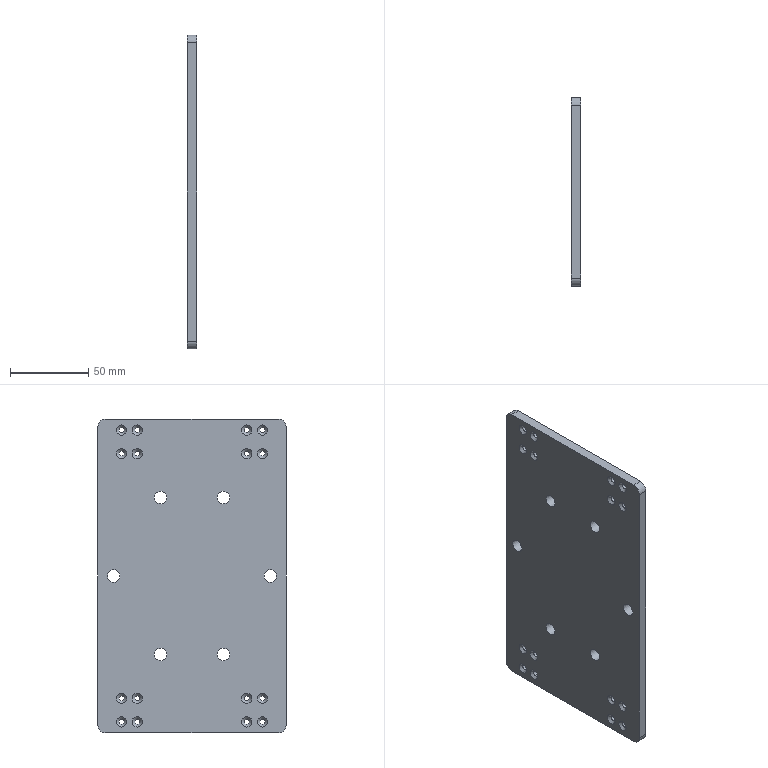Part | STEP file | JBJ-P-1014-02 | 1 solid | 48 faces | box 6 x 120 x 200 mm | volume 140903 mm3 | cylinder 26 | cone 16 | plane 6 | commonest cylinder face diameters 3.4 x16 8 x6 10 x4
STEP:
#1=CARTESIAN_POINT('',(0.,-110.,-96.));
#2=VERTEX_POINT('',#1);
#3=CARTESIAN_POINT('',(0.,-110.,-100.));
#4=DIRECTION('',(-1.,0.,0.));
#5=DIRECTION('',(0.,0.,1.));
#6=AXIS2_PLACEMENT_3D('',#3,#4,#5);
#7=CIRCLE('',#6,4.);
#8=EDGE_CURVE('',#2,#2,#7,.T.);
#9=ORIENTED_EDGE('',*,*,#8,.F.);
#10=EDGE_LOOP('',(#9));
#11=FACE_BOUND('',#10,.T.);
#12=CARTESIAN_POINT('',(0.,-80.,-46.));
#13=VERTEX_POINT('',#12);
#14=CARTESIAN_POINT('',(0.,-80.,-50.));
#15=DIRECTION('',(-1.,0.,0.));
#16=DIRECTION('',(0.,0.,1.));
#17=AXIS2_PLACEMENT_3D('',#14,#15,#16);
#18=CIRCLE('',#17,4.);
#19=EDGE_CURVE('',#13,#13,#18,.T.);
#20=ORIENTED_EDGE('',*,*,#19,.F.);
#21=EDGE_LOOP('',(#20));
#22=FACE_BOUND('',#21,.T.);
#23=CARTESIAN_POINT('',(0.,-40.,-46.));
#24=VERTEX_POINT('',#23);
#25=CARTESIAN_POINT('',(0.,-40.,-50.));
#26=DIRECTION('',(-1.,0.,0.));
#27=DIRECTION('',(0.,0.,1.));
#28=AXIS2_PLACEMENT_3D('',#25,#26,#27);
#29=CIRCLE('',#28,4.);
#30=EDGE_CURVE('',#24,#24,#29,.T.);
#31=ORIENTED_EDGE('',*,*,#30,.F.);
#32=EDGE_LOOP('',(#31));
#33=FACE_BOUND('',#32,.T.);
#34=CARTESIAN_POINT('',(0.,-40.,-146.));
#35=VERTEX_POINT('',#34);
#36=CARTESIAN_POINT('',(0.,-40.,-150.));
#37=DIRECTION('',(-1.,0.,0.));
#38=DIRECTION('',(0.,0.,1.));
#39=AXIS2_PLACEMENT_3D('',#36,#37,#38);
#40=CIRCLE('',#39,4.);
#41=EDGE_CURVE('',#35,#35,#40,.T.);
#42=ORIENTED_EDGE('',*,*,#41,.F.);
#43=EDGE_LOOP('',(#42));
#44=FACE_BOUND('',#43,.T.);
#45=CARTESIAN_POINT('',(0.,-80.,-146.));
#46=VERTEX_POINT('',#45);
#47=CARTESIAN_POINT('',(0.,-80.,-150.));
#48=DIRECTION('',(-1.,0.,0.));
#49=DIRECTION('',(0.,0.,1.));
#50=AXIS2_PLACEMENT_3D('',#47,#48,#49);
#51=CIRCLE('',#50,4.);
#52=EDGE_CURVE('',#46,#46,#51,.T.);
#53=ORIENTED_EDGE('',*,*,#52,.F.);
#54=EDGE_LOOP('',(#53));
#55=FACE_BOUND('',#54,.T.);
#56=CARTESIAN_POINT('',(0.,-104.9,-18.7));
#57=VERTEX_POINT('',#56);
#58=CARTESIAN_POINT('',(0.,-104.9,-22.));
#59=DIRECTION('',(-1.,0.,0.));
#60=DIRECTION('',(0.,0.,1.));
#61=AXIS2_PLACEMENT_3D('',#58,#59,#60);
#62=CIRCLE('',#61,3.3);
#63=EDGE_CURVE('',#57,#57,#62,.T.);
#64=ORIENTED_EDGE('',*,*,#63,.F.);
#65=EDGE_LOOP('',(#64));
#66=FACE_BOUND('',#65,.T.);
#67=CARTESIAN_POINT('',(0.,-104.9,-3.7));
#68=VERTEX_POINT('',#67);
#69=CARTESIAN_POINT('',(0.,-104.9,-7.));
#70=DIRECTION('',(-1.,0.,0.));
#71=DIRECTION('',(0.,0.,1.));
#72=AXIS2_PLACEMENT_3D('',#69,#70,#71);
#73=CIRCLE('',#72,3.3);
#74=EDGE_CURVE('',#68,#68,#73,.T.);
#75=ORIENTED_EDGE('',*,*,#74,.F.);
#76=EDGE_LOOP('',(#75));
#77=FACE_BOUND('',#76,.T.);
#78=CARTESIAN_POINT('',(0.,-94.9,-3.7));
#79=VERTEX_POINT('',#78);
#80=CARTESIAN_POINT('',(0.,-94.9,-7.));
#81=DIRECTION('',(-1.,0.,0.));
#82=DIRECTION('',(0.,0.,1.));
#83=AXIS2_PLACEMENT_3D('',#80,#81,#82);
#84=CIRCLE('',#83,3.3);
#85=EDGE_CURVE('',#79,#79,#84,.T.);
#86=ORIENTED_EDGE('',*,*,#85,.F.);
#87=EDGE_LOOP('',(#86));
#88=FACE_BOUND('',#87,.T.);
#89=CARTESIAN_POINT('',(0.,-25.1,-3.7));
#90=VERTEX_POINT('',#89);
#91=CARTESIAN_POINT('',(0.,-25.1,-7.));
#92=DIRECTION('',(-1.,0.,0.));
#93=DIRECTION('',(0.,0.,1.));
#94=AXIS2_PLACEMENT_3D('',#91,#92,#93);
#95=CIRCLE('',#94,3.3);
#96=EDGE_CURVE('',#90,#90,#95,.T.);
#97=ORIENTED_EDGE('',*,*,#96,.F.);
#98=EDGE_LOOP('',(#97));
#99=FACE_BOUND('',#98,.T.);
#100=CARTESIAN_POINT('',(0.,-15.1,-3.7));
#101=VERTEX_POINT('',#100);
#102=CARTESIAN_POINT('',(0.,-15.1,-7.));
#103=DIRECTION('',(-1.,0.,0.));
#104=DIRECTION('',(0.,0.,1.));
#105=AXIS2_PLACEMENT_3D('',#102,#103,#104);
#106=CIRCLE('',#105,3.3);
#107=EDGE_CURVE('',#101,#101,#106,.T.);
#108=ORIENTED_EDGE('',*,*,#107,.F.);
#109=EDGE_LOOP('',(#108));
#110=FACE_BOUND('',#109,.T.);
#111=CARTESIAN_POINT('',(0.,-25.1,-18.7));
#112=VERTEX_POINT('',#111);
#113=CARTESIAN_POINT('',(0.,-25.1,-22.));
#114=DIRECTION('',(-1.,0.,0.));
#115=DIRECTION('',(0.,0.,1.));
#116=AXIS2_PLACEMENT_3D('',#113,#114,#115);
#117=CIRCLE('',#116,3.3);
#118=EDGE_CURVE('',#112,#112,#117,.T.);
#119=ORIENTED_EDGE('',*,*,#118,.F.);
#120=EDGE_LOOP('',(#119));
#121=FACE_BOUND('',#120,.T.);
#122=CARTESIAN_POINT('',(0.,-15.1,-18.7));
#123=VERTEX_POINT('',#122);
#124=CARTESIAN_POINT('',(0.,-15.1,-22.));
#125=DIRECTION('',(-1.,0.,0.));
#126=DIRECTION('',(0.,0.,1.));
#127=AXIS2_PLACEMENT_3D('',#124,#125,#126);
#128=CIRCLE('',#127,3.3);
#129=EDGE_CURVE('',#123,#123,#128,.T.);
#130=ORIENTED_EDGE('',*,*,#129,.F.);
#131=EDGE_LOOP('',(#130));
#132=FACE_BOUND('',#131,.T.);
#133=CARTESIAN_POINT('',(0.,-104.9,-174.7));
#134=VERTEX_POINT('',#133);
#135=CARTESIAN_POINT('',(0.,-104.9,-178.));
#136=DIRECTION('',(-1.,0.,0.));
#137=DIRECTION('',(0.,0.,1.));
#138=AXIS2_PLACEMENT_3D('',#135,#136,#137);
#139=CIRCLE('',#138,3.3);
#140=EDGE_CURVE('',#134,#134,#139,.T.);
#141=ORIENTED_EDGE('',*,*,#140,.F.);
#142=EDGE_LOOP('',(#141));
#143=FACE_BOUND('',#142,.T.);
#144=CARTESIAN_POINT('',(0.,-104.9,-189.7));
#145=VERTEX_POINT('',#144);
#146=CARTESIAN_POINT('',(0.,-104.9,-193.));
#147=DIRECTION('',(-1.,0.,0.));
#148=DIRECTION('',(0.,0.,1.));
#149=AXIS2_PLACEMENT_3D('',#146,#147,#148);
#150=CIRCLE('',#149,3.3);
#151=EDGE_CURVE('',#145,#145,#150,.T.);
#152=ORIENTED_EDGE('',*,*,#151,.F.);
#153=EDGE_LOOP('',(#152));
#154=FACE_BOUND('',#153,.T.);
#155=CARTESIAN_POINT('',(0.,-94.9,-189.7));
#156=VERTEX_POINT('',#155);
#157=CARTESIAN_POINT('',(0.,-94.9,-193.));
#158=DIRECTION('',(-1.,0.,0.));
#159=DIRECTION('',(0.,0.,1.));
#160=AXIS2_PLACEMENT_3D('',#157,#158,#159);
#161=CIRCLE('',#160,3.3);
#162=EDGE_CURVE('',#156,#156,#161,.T.);
#163=ORIENTED_EDGE('',*,*,#162,.F.);
#164=EDGE_LOOP('',(#163));
#165=FACE_BOUND('',#164,.T.);
#166=CARTESIAN_POINT('',(0.,-94.9,-174.7));
#167=VERTEX_POINT('',#166);
#168=CARTESIAN_POINT('',(0.,-94.9,-178.));
#169=DIRECTION('',(-1.,0.,0.));
#170=DIRECTION('',(0.,0.,1.));
#171=AXIS2_PLACEMENT_3D('',#168,#169,#170);
#172=CIRCLE('',#171,3.3);
#173=EDGE_CURVE('',#167,#167,#172,.T.);
#174=ORIENTED_EDGE('',*,*,#173,.F.);
#175=EDGE_LOOP('',(#174));
#176=FACE_BOUND('',#175,.T.);
#177=CARTESIAN_POINT('',(0.,-25.1,-174.7));
#178=VERTEX_POINT('',#177);
#179=CARTESIAN_POINT('',(0.,-25.1,-178.));
#180=DIRECTION('',(-1.,0.,0.));
#181=DIRECTION('',(0.,0.,1.));
#182=AXIS2_PLACEMENT_3D('',#179,#180,#181);
#183=CIRCLE('',#182,3.3);
#184=EDGE_CURVE('',#178,#178,#183,.T.);
#185=ORIENTED_EDGE('',*,*,#184,.F.);
#186=EDGE_LOOP('',(#185));
#187=FACE_BOUND('',#186,.T.);
#188=CARTESIAN_POINT('',(0.,-15.1,-174.7));
#189=VERTEX_POINT('',#188);
#190=CARTESIAN_POINT('',(0.,-15.1,-178.));
#191=DIRECTION('',(-1.,0.,0.));
#192=DIRECTION('',(0.,0.,1.));
#193=AXIS2_PLACEMENT_3D('',#190,#191,#192);
#194=CIRCLE('',#193,3.3);
#195=EDGE_CURVE('',#189,#189,#194,.T.);
#196=ORIENTED_EDGE('',*,*,#195,.F.);
#197=EDGE_LOOP('',(#196));
#198=FACE_BOUND('',#197,.T.);
#199=CARTESIAN_POINT('',(0.,-15.1,-189.7));
#200=VERTEX_POINT('',#199);
#201=CARTESIAN_POINT('',(0.,-15.1,-193.));
#202=DIRECTION('',(-1.,0.,0.));
#203=DIRECTION('',(0.,0.,1.));
#204=AXIS2_PLACEMENT_3D('',#201,#202,#203);
#205=CIRCLE('',#204,3.3);
#206=EDGE_CURVE('',#200,#200,#205,.T.);
#207=ORIENTED_EDGE('',*,*,#206,.F.);
#208=EDGE_LOOP('',(#207));
#209=FACE_BOUND('',#208,.T.);
#210=CARTESIAN_POINT('',(0.,-25.1,-189.7));
#211=VERTEX_POINT('',#210);
#212=CARTESIAN_POINT('',(0.,-25.1,-193.));
#213=DIRECTION('',(-1.,0.,0.));
#214=DIRECTION('',(0.,0.,1.));
#215=AXIS2_PLACEMENT_3D('',#212,#213,#214);
#216=CIRCLE('',#215,3.3);
#217=EDGE_CURVE('',#211,#211,#216,.T.);
#218=ORIENTED_EDGE('',*,*,#217,.F.);
#219=EDGE_LOOP('',(#218));
#220=FACE_BOUND('',#219,.T.);
#221=CARTESIAN_POINT('',(0.,-120.,-5.));
#222=VERTEX_POINT('',#221);
#223=CARTESIAN_POINT('',(0.,-120.,-195.));
#224=VERTEX_POINT('',#223);
#225=CARTESIAN_POINT('',(0.,-120.,0.));
#226=DIRECTION('',(0.,0.,-1.));
#227=VECTOR('',#226,1000.);
#228=LINE('',#225,#227);
#229=EDGE_CURVE('',#222,#224,#228,.T.);
#230=ORIENTED_EDGE('',*,*,#229,.F.);
#231=CARTESIAN_POINT('',(0.,-115.,0.));
#232=VERTEX_POINT('',#231);
#233=CARTESIAN_POINT('',(0.,-115.,-5.));
#234=DIRECTION('',(-1.,0.,0.));
#235=DIRECTION('',(0.,0.,-1.));
#236=AXIS2_PLACEMENT_3D('',#233,#234,#235);
#237=CIRCLE('',#236,5.);
#238=EDGE_CURVE('',#222,#232,#237,.T.);
#239=ORIENTED_EDGE('',*,*,#238,.T.);
#240=CARTESIAN_POINT('',(0.,-5.,0.));
#241=VERTEX_POINT('',#240);
#242=CARTESIAN_POINT('',(0.,0.,0.));
#243=DIRECTION('',(0.,-1.,0.));
#244=VECTOR('',#243,1000.);
#245=LINE('',#242,#244);
#246=EDGE_CURVE('',#241,#232,#245,.T.);
#247=ORIENTED_EDGE('',*,*,#246,.F.);
#248=CARTESIAN_POINT('',(0.,0.,-5.));
#249=VERTEX_POINT('',#248);
#250=CARTESIAN_POINT('',(0.,-5.,-5.));
#251=DIRECTION('',(-1.,0.,0.));
#252=DIRECTION('',(0.,0.,-1.));
#253=AXIS2_PLACEMENT_3D('',#250,#251,#252);
#254=CIRCLE('',#253,5.);
#255=EDGE_CURVE('',#241,#249,#254,.T.);
#256=ORIENTED_EDGE('',*,*,#255,.T.);
#257=CARTESIAN_POINT('',(0.,0.,-195.));
#258=VERTEX_POINT('',#257);
#259=CARTESIAN_POINT('',(0.,0.,0.));
#260=DIRECTION('',(0.,0.,1.));
#261=VECTOR('',#260,1000.);
#262=LINE('',#259,#261);
#263=EDGE_CURVE('',#258,#249,#262,.T.);
#264=ORIENTED_EDGE('',*,*,#263,.F.);
#265=CARTESIAN_POINT('',(0.,-5.,-200.));
#266=VERTEX_POINT('',#265);
#267=CARTESIAN_POINT('',(0.,-5.,-195.));
#268=DIRECTION('',(-1.,0.,0.));
#269=DIRECTION('',(0.,0.,-1.));
#270=AXIS2_PLACEMENT_3D('',#267,#268,#269);
#271=CIRCLE('',#270,5.);
#272=EDGE_CURVE('',#258,#266,#271,.T.);
#273=ORIENTED_EDGE('',*,*,#272,.T.);
#274=CARTESIAN_POINT('',(0.,-115.,-200.));
#275=VERTEX_POINT('',#274);
#276=CARTESIAN_POINT('',(0.,0.,-200.));
#277=DIRECTION('',(0.,1.,0.));
#278=VECTOR('',#277,1000.);
#279=LINE('',#276,#278);
#280=EDGE_CURVE('',#275,#266,#279,.T.);
#281=ORIENTED_EDGE('',*,*,#280,.F.);
#282=CARTESIAN_POINT('',(0.,-115.,-195.));
#283=DIRECTION('',(-1.,0.,0.));
#284=DIRECTION('',(0.,0.,-1.));
#285=AXIS2_PLACEMENT_3D('',#282,#283,#284);
#286=CIRCLE('',#285,5.);
#287=EDGE_CURVE('',#275,#224,#286,.T.);
#288=ORIENTED_EDGE('',*,*,#287,.T.);
#289=EDGE_LOOP('',(#230,#239,#247,#256,#264,#273,#281,#288));
#290=FACE_OUTER_BOUND('',#289,.T.);
#291=CARTESIAN_POINT('',(0.,-94.9,-18.7));
#292=VERTEX_POINT('',#291);
#293=CARTESIAN_POINT('',(0.,-94.9,-22.));
#294=DIRECTION('',(-1.,0.,0.));
#295=DIRECTION('',(0.,0.,1.));
#296=AXIS2_PLACEMENT_3D('',#293,#294,#295);
#297=CIRCLE('',#296,3.3);
#298=EDGE_CURVE('',#292,#292,#297,.T.);
#299=ORIENTED_EDGE('',*,*,#298,.F.);
#300=EDGE_LOOP('',(#299));
#301=FACE_BOUND('',#300,.T.);
#302=CARTESIAN_POINT('',(0.,-10.,-96.));
#303=VERTEX_POINT('',#302);
#304=CARTESIAN_POINT('',(0.,-10.,-100.));
#305=DIRECTION('',(-1.,0.,0.));
#306=DIRECTION('',(0.,0.,1.));
#307=AXIS2_PLACEMENT_3D('',#304,#305,#306);
#308=CIRCLE('',#307,4.);
#309=EDGE_CURVE('',#303,#303,#308,.T.);
#310=ORIENTED_EDGE('',*,*,#309,.F.);
#311=EDGE_LOOP('',(#310));
#312=FACE_BOUND('',#311,.T.);
#313=CARTESIAN_POINT('',(0.,0.,0.));
#314=DIRECTION('',(1.,0.,0.));
#315=DIRECTION('',(0.,0.,-1.));
#316=AXIS2_PLACEMENT_3D('',#313,#314,#315);
#317=PLANE('',#316);
#318=ADVANCED_FACE('',(#11,#22,#33,#44,#55,#66,#77,#88,#99,#110,#121,#132,#143,#154,#165,#176,#187,#198,#209,#220,#290,#301,#312),#317,.F.);
#319=ORIENTED_EDGE('',*,*,#246,.T.);
#320=CARTESIAN_POINT('',(6.,-115.,0.));
#321=VERTEX_POINT('',#320);
#322=CARTESIAN_POINT('',(6.,-115.,0.));
#323=DIRECTION('',(1.,0.,0.));
#324=VECTOR('',#323,1000.);
#325=LINE('',#322,#324);
#326=EDGE_CURVE('',#232,#321,#325,.T.);
#327=ORIENTED_EDGE('',*,*,#326,.T.);
#328=CARTESIAN_POINT('',(6.,-5.,0.));
#329=VERTEX_POINT('',#328);
#330=CARTESIAN_POINT('',(6.,0.,0.));
#331=DIRECTION('',(0.,-1.,0.));
#332=VECTOR('',#331,1000.);
#333=LINE('',#330,#332);
#334=EDGE_CURVE('',#329,#321,#333,.T.);
#335=ORIENTED_EDGE('',*,*,#334,.F.);
#336=CARTESIAN_POINT('',(6.,-5.,0.));
#337=DIRECTION('',(-1.,0.,0.));
#338=VECTOR('',#337,1000.);
#339=LINE('',#336,#338);
#340=EDGE_CURVE('',#329,#241,#339,.T.);
#341=ORIENTED_EDGE('',*,*,#340,.T.);
#342=EDGE_LOOP('',(#319,#327,#335,#341));
#343=FACE_OUTER_BOUND('',#342,.T.);
#344=CARTESIAN_POINT('',(6.,0.,0.));
#345=DIRECTION('',(0.,0.,-1.));
#346=DIRECTION('',(0.,1.,0.));
#347=AXIS2_PLACEMENT_3D('',#344,#345,#346);
#348=PLANE('',#347);
#349=ADVANCED_FACE('',(#343),#348,.F.);
#350=CARTESIAN_POINT('',(6.,-120.,-5.));
#351=VERTEX_POINT('',#350);
#352=CARTESIAN_POINT('',(6.,-120.,-195.));
#353=VERTEX_POINT('',#352);
#354=CARTESIAN_POINT('',(6.,-120.,0.));
#355=DIRECTION('',(0.,0.,-1.));
#356=VECTOR('',#355,1000.);
#357=LINE('',#354,#356);
#358=EDGE_CURVE('',#351,#353,#357,.T.);
#359=ORIENTED_EDGE('',*,*,#358,.F.);
#360=CARTESIAN_POINT('',(6.,-120.,-5.));
#361=DIRECTION('',(-1.,0.,0.));
#362=VECTOR('',#361,1000.);
#363=LINE('',#360,#362);
#364=EDGE_CURVE('',#351,#222,#363,.T.);
#365=ORIENTED_EDGE('',*,*,#364,.T.);
#366=ORIENTED_EDGE('',*,*,#229,.T.);
#367=CARTESIAN_POINT('',(6.,-120.,-195.));
#368=DIRECTION('',(1.,0.,0.));
#369=VECTOR('',#368,1000.);
#370=LINE('',#367,#369);
#371=EDGE_CURVE('',#224,#353,#370,.T.);
#372=ORIENTED_EDGE('',*,*,#371,.T.);
#373=EDGE_LOOP('',(#359,#365,#366,#372));
#374=FACE_OUTER_BOUND('',#373,.T.);
#375=CARTESIAN_POINT('',(6.,-120.,0.));
#376=DIRECTION('',(0.,1.,0.));
#377=DIRECTION('',(0.,0.,1.));
#378=AXIS2_PLACEMENT_3D('',#375,#376,#377);
#379=PLANE('',#378);
#380=ADVANCED_FACE('',(#374),#379,.F.);
#381=CARTESIAN_POINT('',(6.,-115.,-200.));
#382=VERTEX_POINT('',#381);
#383=CARTESIAN_POINT('',(6.,-5.,-200.));
#384=VERTEX_POINT('',#383);
#385=CARTESIAN_POINT('',(6.,0.,-200.));
#386=DIRECTION('',(0.,1.,0.));
#387=VECTOR('',#386,1000.);
#388=LINE('',#385,#387);
#389=EDGE_CURVE('',#382,#384,#388,.T.);
#390=ORIENTED_EDGE('',*,*,#389,.F.);
#391=CARTESIAN_POINT('',(6.,-115.,-200.));
#392=DIRECTION('',(-1.,0.,0.));
#393=VECTOR('',#392,1000.);
#394=LINE('',#391,#393);
#395=EDGE_CURVE('',#382,#275,#394,.T.);
#396=ORIENTED_EDGE('',*,*,#395,.T.);
#397=ORIENTED_EDGE('',*,*,#280,.T.);
#398=CARTESIAN_POINT('',(6.,-5.,-200.));
#399=DIRECTION('',(1.,0.,0.));
#400=VECTOR('',#399,1000.);
#401=LINE('',#398,#400);
#402=EDGE_CURVE('',#266,#384,#401,.T.);
#403=ORIENTED_EDGE('',*,*,#402,.T.);
#404=EDGE_LOOP('',(#390,#396,#397,#403));
#405=FACE_OUTER_BOUND('',#404,.T.);
#406=CARTESIAN_POINT('',(6.,0.,-200.));
#407=DIRECTION('',(0.,0.,1.));
#408=DIRECTION('',(0.,-1.,0.));
#409=AXIS2_PLACEMENT_3D('',#406,#407,#408);
#410=PLANE('',#409);
#411=ADVANCED_FACE('',(#405),#410,.F.);
#412=CARTESIAN_POINT('',(6.,0.,-195.));
#413=VERTEX_POINT('',#412);
#414=CARTESIAN_POINT('',(6.,0.,-5.));
#415=VERTEX_POINT('',#414);
#416=CARTESIAN_POINT('',(6.,0.,0.));
#417=DIRECTION('',(0.,0.,1.));
#418=VECTOR('',#417,1000.);
#419=LINE('',#416,#418);
#420=EDGE_CURVE('',#413,#415,#419,.T.);
#421=ORIENTED_EDGE('',*,*,#420,.F.);
#422=CARTESIAN_POINT('',(6.,0.,-195.));
#423=DIRECTION('',(-1.,0.,0.));
#424=VECTOR('',#423,1000.);
#425=LINE('',#422,#424);
#426=EDGE_CURVE('',#413,#258,#425,.T.);
#427=ORIENTED_EDGE('',*,*,#426,.T.);
#428=ORIENTED_EDGE('',*,*,#263,.T.);
#429=CARTESIAN_POINT('',(6.,0.,-5.));
#430=DIRECTION('',(1.,0.,0.));
#431=VECTOR('',#430,1000.);
#432=LINE('',#429,#431);
#433=EDGE_CURVE('',#249,#415,#432,.T.);
#434=ORIENTED_EDGE('',*,*,#433,.T.);
#435=EDGE_LOOP('',(#421,#427,#428,#434));
#436=FACE_OUTER_BOUND('',#435,.T.);
#437=CARTESIAN_POINT('',(6.,0.,0.));
#438=DIRECTION('',(0.,-1.,0.));
#439=DIRECTION('',(0.,0.,-1.));
#440=AXIS2_PLACEMENT_3D('',#437,#438,#439);
#441=PLANE('',#440);
#442=ADVANCED_FACE('',(#436),#441,.F.);
#443=CARTESIAN_POINT('',(6.,-10.,-96.));
#444=VERTEX_POINT('',#443);
#445=CARTESIAN_POINT('',(6.,-10.,-100.));
#446=DIRECTION('',(-1.,0.,0.));
#447=DIRECTION('',(0.,0.,1.));
#448=AXIS2_PLACEMENT_3D('',#445,#446,#447);
#449=CIRCLE('',#448,4.);
#450=EDGE_CURVE('',#444,#444,#449,.T.);
#451=ORIENTED_EDGE('',*,*,#450,.T.);
#452=EDGE_LOOP('',(#451));
#453=FACE_BOUND('',#452,.T.);
#454=CARTESIAN_POINT('',(6.,-110.,-96.));
#455=VERTEX_POINT('',#454);
#456=CARTESIAN_POINT('',(6.,-110.,-100.));
#457=DIRECTION('',(-1.,0.,0.));
#458=DIRECTION('',(0.,0.,1.));
#459=AXIS2_PLACEMENT_3D('',#456,#457,#458);
#460=CIRCLE('',#459,4.);
#461=EDGE_CURVE('',#455,#455,#460,.T.);
#462=ORIENTED_EDGE('',*,*,#461,.T.);
#463=EDGE_LOOP('',(#462));
#464=FACE_BOUND('',#463,.T.);
#465=CARTESIAN_POINT('',(6.,-80.,-46.));
#466=VERTEX_POINT('',#465);
#467=CARTESIAN_POINT('',(6.,-80.,-50.));
#468=DIRECTION('',(-1.,0.,0.));
#469=DIRECTION('',(0.,0.,1.));
#470=AXIS2_PLACEMENT_3D('',#467,#468,#469);
#471=CIRCLE('',#470,4.);
#472=EDGE_CURVE('',#466,#466,#471,.T.);
#473=ORIENTED_EDGE('',*,*,#472,.T.);
#474=EDGE_LOOP('',(#473));
#475=FACE_BOUND('',#474,.T.);
#476=CARTESIAN_POINT('',(6.,-40.,-46.));
#477=VERTEX_POINT('',#476);
#478=CARTESIAN_POINT('',(6.,-40.,-50.));
#479=DIRECTION('',(-1.,0.,0.));
#480=DIRECTION('',(0.,0.,1.));
#481=AXIS2_PLACEMENT_3D('',#478,#479,#480);
#482=CIRCLE('',#481,4.);
#483=EDGE_CURVE('',#477,#477,#482,.T.);
#484=ORIENTED_EDGE('',*,*,#483,.T.);
#485=EDGE_LOOP('',(#484));
#486=FACE_BOUND('',#485,.T.);
#487=CARTESIAN_POINT('',(6.,-40.,-146.));
#488=VERTEX_POINT('',#487);
#489=CARTESIAN_POINT('',(6.,-40.,-150.));
#490=DIRECTION('',(-1.,0.,0.));
#491=DIRECTION('',(0.,0.,1.));
#492=AXIS2_PLACEMENT_3D('',#489,#490,#491);
#493=CIRCLE('',#492,4.);
#494=EDGE_CURVE('',#488,#488,#493,.T.);
#495=ORIENTED_EDGE('',*,*,#494,.T.);
#496=EDGE_LOOP('',(#495));
#497=FACE_BOUND('',#496,.T.);
#498=CARTESIAN_POINT('',(6.,-80.,-146.));
#499=VERTEX_POINT('',#498);
#500=CARTESIAN_POINT('',(6.,-80.,-150.));
#501=DIRECTION('',(-1.,0.,0.));
#502=DIRECTION('',(0.,0.,1.));
#503=AXIS2_PLACEMENT_3D('',#500,#501,#502);
#504=CIRCLE('',#503,4.);
#505=EDGE_CURVE('',#499,#499,#504,.T.);
#506=ORIENTED_EDGE('',*,*,#505,.T.);
#507=EDGE_LOOP('',(#506));
#508=FACE_BOUND('',#507,.T.);
#509=CARTESIAN_POINT('',(6.,-104.9,-20.3));
#510=VERTEX_POINT('',#509);
#511=CARTESIAN_POINT('',(6.,-104.9,-22.));
#512=DIRECTION('',(-1.,0.,0.));
#513=DIRECTION('',(0.,0.,1.));
#514=AXIS2_PLACEMENT_3D('',#511,#512,#513);
#515=CIRCLE('',#514,1.7);
#516=EDGE_CURVE('',#510,#510,#515,.T.);
#517=ORIENTED_EDGE('',*,*,#516,.T.);
#518=EDGE_LOOP('',(#517));
#519=FACE_BOUND('',#518,.T.);
#520=CARTESIAN_POINT('',(6.,-104.9,-5.3));
#521=VERTEX_POINT('',#520);
#522=CARTESIAN_POINT('',(6.,-104.9,-7.));
#523=DIRECTION('',(-1.,0.,0.));
#524=DIRECTION('',(0.,0.,1.));
#525=AXIS2_PLACEMENT_3D('',#522,#523,#524);
#526=CIRCLE('',#525,1.7);
#527=EDGE_CURVE('',#521,#521,#526,.T.);
#528=ORIENTED_EDGE('',*,*,#527,.T.);
#529=EDGE_LOOP('',(#528));
#530=FACE_BOUND('',#529,.T.);
#531=CARTESIAN_POINT('',(6.,-94.9,-5.3));
#532=VERTEX_POINT('',#531);
#533=CARTESIAN_POINT('',(6.,-94.9,-7.));
#534=DIRECTION('',(-1.,0.,0.));
#535=DIRECTION('',(0.,0.,1.));
#536=AXIS2_PLACEMENT_3D('',#533,#534,#535);
#537=CIRCLE('',#536,1.7);
#538=EDGE_CURVE('',#532,#532,#537,.T.);
#539=ORIENTED_EDGE('',*,*,#538,.T.);
#540=EDGE_LOOP('',(#539));
#541=FACE_BOUND('',#540,.T.);
#542=CARTESIAN_POINT('',(6.,-94.9,-20.3));
#543=VERTEX_POINT('',#542);
#544=CARTESIAN_POINT('',(6.,-94.9,-22.));
#545=DIRECTION('',(-1.,0.,0.));
#546=DIRECTION('',(0.,0.,1.));
#547=AXIS2_PLACEMENT_3D('',#544,#545,#546);
#548=CIRCLE('',#547,1.7);
#549=EDGE_CURVE('',#543,#543,#548,.T.);
#550=ORIENTED_EDGE('',*,*,#549,.T.);
#551=EDGE_LOOP('',(#550));
#552=FACE_BOUND('',#551,.T.);
#553=CARTESIAN_POINT('',(6.,-25.1,-5.3));
#554=VERTEX_POINT('',#553);
#555=CARTESIAN_POINT('',(6.,-25.1,-7.));
#556=DIRECTION('',(-1.,0.,0.));
#557=DIRECTION('',(0.,0.,1.));
#558=AXIS2_PLACEMENT_3D('',#555,#556,#557);
#559=CIRCLE('',#558,1.7);
#560=EDGE_CURVE('',#554,#554,#559,.T.);
#561=ORIENTED_EDGE('',*,*,#560,.T.);
#562=EDGE_LOOP('',(#561));
#563=FACE_BOUND('',#562,.T.);
#564=CARTESIAN_POINT('',(6.,-15.1,-5.3));
#565=VERTEX_POINT('',#564);
#566=CARTESIAN_POINT('',(6.,-15.1,-7.));
#567=DIRECTION('',(-1.,0.,0.));
#568=DIRECTION('',(0.,0.,1.));
#569=AXIS2_PLACEMENT_3D('',#566,#567,#568);
#570=CIRCLE('',#569,1.7);
#571=EDGE_CURVE('',#565,#565,#570,.T.);
#572=ORIENTED_EDGE('',*,*,#571,.T.);
#573=EDGE_LOOP('',(#572));
#574=FACE_BOUND('',#573,.T.);
#575=CARTESIAN_POINT('',(6.,-25.1,-20.3));
#576=VERTEX_POINT('',#575);
#577=CARTESIAN_POINT('',(6.,-25.1,-22.));
#578=DIRECTION('',(-1.,0.,0.));
#579=DIRECTION('',(0.,0.,1.));
#580=AXIS2_PLACEMENT_3D('',#577,#578,#579);
#581=CIRCLE('',#580,1.7);
#582=EDGE_CURVE('',#576,#576,#581,.T.);
#583=ORIENTED_EDGE('',*,*,#582,.T.);
#584=EDGE_LOOP('',(#583));
#585=FACE_BOUND('',#584,.T.);
#586=CARTESIAN_POINT('',(6.,-15.1,-20.3));
#587=VERTEX_POINT('',#586);
#588=CARTESIAN_POINT('',(6.,-15.1,-22.));
#589=DIRECTION('',(-1.,0.,0.));
#590=DIRECTION('',(0.,0.,1.));
#591=AXIS2_PLACEMENT_3D('',#588,#589,#590);
#592=CIRCLE('',#591,1.7);
#593=EDGE_CURVE('',#587,#587,#592,.T.);
#594=ORIENTED_EDGE('',*,*,#593,.T.);
#595=EDGE_LOOP('',(#594));
#596=FACE_BOUND('',#595,.T.);
#597=CARTESIAN_POINT('',(6.,-104.9,-176.3));
#598=VERTEX_POINT('',#597);
#599=CARTESIAN_POINT('',(6.,-104.9,-178.));
#600=DIRECTION('',(-1.,0.,0.));
#601=DIRECTION('',(0.,0.,1.));
#602=AXIS2_PLACEMENT_3D('',#599,#600,#601);
#603=CIRCLE('',#602,1.7);
#604=EDGE_CURVE('',#598,#598,#603,.T.);
#605=ORIENTED_EDGE('',*,*,#604,.T.);
#606=EDGE_LOOP('',(#605));
#607=FACE_BOUND('',#606,.T.);
#608=CARTESIAN_POINT('',(6.,-104.9,-191.3));
#609=VERTEX_POINT('',#608);
#610=CARTESIAN_POINT('',(6.,-104.9,-193.));
#611=DIRECTION('',(-1.,0.,0.));
#612=DIRECTION('',(0.,0.,1.));
#613=AXIS2_PLACEMENT_3D('',#610,#611,#612);
#614=CIRCLE('',#613,1.7);
#615=EDGE_CURVE('',#609,#609,#614,.T.);
#616=ORIENTED_EDGE('',*,*,#615,.T.);
#617=EDGE_LOOP('',(#616));
#618=FACE_BOUND('',#617,.T.);
#619=CARTESIAN_POINT('',(6.,-94.9,-191.3));
#620=VERTEX_POINT('',#619);
#621=CARTESIAN_POINT('',(6.,-94.9,-193.));
#622=DIRECTION('',(-1.,0.,0.));
#623=DIRECTION('',(0.,0.,1.));
#624=AXIS2_PLACEMENT_3D('',#621,#622,#623);
#625=CIRCLE('',#624,1.7);
#626=EDGE_CURVE('',#620,#620,#625,.T.);
#627=ORIENTED_EDGE('',*,*,#626,.T.);
#628=EDGE_LOOP('',(#627));
#629=FACE_BOUND('',#628,.T.);
#630=CARTESIAN_POINT('',(6.,-94.9,-176.3));
#631=VERTEX_POINT('',#630);
#632=CARTESIAN_POINT('',(6.,-94.9,-178.));
#633=DIRECTION('',(-1.,0.,0.));
#634=DIRECTION('',(0.,0.,1.));
#635=AXIS2_PLACEMENT_3D('',#632,#633,#634);
#636=CIRCLE('',#635,1.7);
#637=EDGE_CURVE('',#631,#631,#636,.T.);
#638=ORIENTED_EDGE('',*,*,#637,.T.);
#639=EDGE_LOOP('',(#638));
#640=FACE_BOUND('',#639,.T.);
#641=CARTESIAN_POINT('',(6.,-25.1,-176.3));
#642=VERTEX_POINT('',#641);
#643=CARTESIAN_POINT('',(6.,-25.1,-178.));
#644=DIRECTION('',(-1.,0.,0.));
#645=DIRECTION('',(0.,0.,1.));
#646=AXIS2_PLACEMENT_3D('',#643,#644,#645);
#647=CIRCLE('',#646,1.7);
#648=EDGE_CURVE('',#642,#642,#647,.T.);
#649=ORIENTED_EDGE('',*,*,#648,.T.);
#650=EDGE_LOOP('',(#649));
#651=FACE_BOUND('',#650,.T.);
#652=CARTESIAN_POINT('',(6.,-15.1,-176.3));
#653=VERTEX_POINT('',#652);
#654=CARTESIAN_POINT('',(6.,-15.1,-178.));
#655=DIRECTION('',(-1.,0.,0.));
#656=DIRECTION('',(0.,0.,1.));
#657=AXIS2_PLACEMENT_3D('',#654,#655,#656);
#658=CIRCLE('',#657,1.7);
#659=EDGE_CURVE('',#653,#653,#658,.T.);
#660=ORIENTED_EDGE('',*,*,#659,.T.);
#661=EDGE_LOOP('',(#660));
#662=FACE_BOUND('',#661,.T.);
#663=CARTESIAN_POINT('',(6.,-15.1,-191.3));
#664=VERTEX_POINT('',#663);
#665=CARTESIAN_POINT('',(6.,-15.1,-193.));
#666=DIRECTION('',(-1.,0.,0.));
#667=DIRECTION('',(0.,0.,1.));
#668=AXIS2_PLACEMENT_3D('',#665,#666,#667);
#669=CIRCLE('',#668,1.7);
#670=EDGE_CURVE('',#664,#664,#669,.T.);
#671=ORIENTED_EDGE('',*,*,#670,.T.);
#672=EDGE_LOOP('',(#671));
#673=FACE_BOUND('',#672,.T.);
#674=CARTESIAN_POINT('',(6.,-25.1,-191.3));
#675=VERTEX_POINT('',#674);
#676=CARTESIAN_POINT('',(6.,-25.1,-193.));
#677=DIRECTION('',(-1.,0.,0.));
#678=DIRECTION('',(0.,0.,1.));
#679=AXIS2_PLACEMENT_3D('',#676,#677,#678);
#680=CIRCLE('',#679,1.7);
#681=EDGE_CURVE('',#675,#675,#680,.T.);
#682=ORIENTED_EDGE('',*,*,#681,.T.);
#683=EDGE_LOOP('',(#682));
#684=FACE_BOUND('',#683,.T.);
#685=ORIENTED_EDGE('',*,*,#334,.T.);
#686=CARTESIAN_POINT('',(6.,-115.,-5.));
#687=DIRECTION('',(1.,0.,0.));
#688=DIRECTION('',(0.,0.,-1.));
#689=AXIS2_PLACEMENT_3D('',#686,#687,#688);
#690=CIRCLE('',#689,5.);
#691=EDGE_CURVE('',#321,#351,#690,.T.);
#692=ORIENTED_EDGE('',*,*,#691,.T.);
#693=ORIENTED_EDGE('',*,*,#358,.T.);
#694=CARTESIAN_POINT('',(6.,-115.,-195.));
#695=DIRECTION('',(1.,0.,0.));
#696=DIRECTION('',(0.,0.,-1.));
#697=AXIS2_PLACEMENT_3D('',#694,#695,#696);
#698=CIRCLE('',#697,5.);
#699=EDGE_CURVE('',#353,#382,#698,.T.);
#700=ORIENTED_EDGE('',*,*,#699,.T.);
#701=ORIENTED_EDGE('',*,*,#389,.T.);
#702=CARTESIAN_POINT('',(6.,-5.,-195.));
#703=DIRECTION('',(1.,0.,0.));
#704=DIRECTION('',(0.,0.,-1.));
#705=AXIS2_PLACEMENT_3D('',#702,#703,#704);
#706=CIRCLE('',#705,5.);
#707=EDGE_CURVE('',#384,#413,#706,.T.);
#708=ORIENTED_EDGE('',*,*,#707,.T.);
#709=ORIENTED_EDGE('',*,*,#420,.T.);
#710=CARTESIAN_POINT('',(6.,-5.,-5.));
#711=DIRECTION('',(1.,0.,0.));
#712=DIRECTION('',(0.,0.,-1.));
#713=AXIS2_PLACEMENT_3D('',#710,#711,#712);
#714=CIRCLE('',#713,5.);
#715=EDGE_CURVE('',#415,#329,#714,.T.);
#716=ORIENTED_EDGE('',*,*,#715,.T.);
#717=EDGE_LOOP('',(#685,#692,#693,#700,#701,#708,#709,#716));
#718=FACE_OUTER_BOUND('',#717,.T.);
#719=CARTESIAN_POINT('',(6.,0.,0.));
#720=DIRECTION('',(1.,0.,0.));
#721=DIRECTION('',(0.,0.,-1.));
#722=AXIS2_PLACEMENT_3D('',#719,#720,#721);
#723=PLANE('',#722);
#724=ADVANCED_FACE('',(#453,#464,#475,#486,#497,#508,#519,#530,#541,#552,#563,#574,#585,#596,#607,#618,#629,#640,#651,#662,#673,#684,#718),#723,.T.);
#725=ORIENTED_EDGE('',*,*,#691,.F.);
#726=ORIENTED_EDGE('',*,*,#326,.F.);
#727=ORIENTED_EDGE('',*,*,#238,.F.);
#728=ORIENTED_EDGE('',*,*,#364,.F.);
#729=EDGE_LOOP('',(#725,#726,#727,#728));
#730=FACE_OUTER_BOUND('',#729,.T.);
#731=CARTESIAN_POINT('',(6.,-115.,-5.));
#732=DIRECTION('',(-1.,0.,0.));
#733=DIRECTION('',(0.,0.,1.));
#734=AXIS2_PLACEMENT_3D('',#731,#732,#733);
#735=CYLINDRICAL_SURFACE('',#734,5.);
#736=ADVANCED_FACE('',(#730),#735,.T.);
#737=ORIENTED_EDGE('',*,*,#699,.F.);
#738=ORIENTED_EDGE('',*,*,#371,.F.);
#739=ORIENTED_EDGE('',*,*,#287,.F.);
#740=ORIENTED_EDGE('',*,*,#395,.F.);
#741=EDGE_LOOP('',(#737,#738,#739,#740));
#742=FACE_OUTER_BOUND('',#741,.T.);
#743=CARTESIAN_POINT('',(6.,-115.,-195.));
#744=DIRECTION('',(-1.,0.,0.));
#745=DIRECTION('',(0.,0.,1.));
#746=AXIS2_PLACEMENT_3D('',#743,#744,#745);
#747=CYLINDRICAL_SURFACE('',#746,5.);
#748=ADVANCED_FACE('',(#742),#747,.T.);
#749=ORIENTED_EDGE('',*,*,#707,.F.);
#750=ORIENTED_EDGE('',*,*,#402,.F.);
#751=ORIENTED_EDGE('',*,*,#272,.F.);
#752=ORIENTED_EDGE('',*,*,#426,.F.);
#753=EDGE_LOOP('',(#749,#750,#751,#752));
#754=FACE_OUTER_BOUND('',#753,.T.);
#755=CARTESIAN_POINT('',(6.,-5.,-195.));
#756=DIRECTION('',(-1.,0.,0.));
#757=DIRECTION('',(0.,0.,1.));
#758=AXIS2_PLACEMENT_3D('',#755,#756,#757);
#759=CYLINDRICAL_SURFACE('',#758,5.);
#760=ADVANCED_FACE('',(#754),#759,.T.);
#761=ORIENTED_EDGE('',*,*,#715,.F.);
#762=ORIENTED_EDGE('',*,*,#433,.F.);
#763=ORIENTED_EDGE('',*,*,#255,.F.);
#764=ORIENTED_EDGE('',*,*,#340,.F.);
#765=EDGE_LOOP('',(#761,#762,#763,#764));
#766=FACE_OUTER_BOUND('',#765,.T.);
#767=CARTESIAN_POINT('',(6.,-5.,-5.));
#768=DIRECTION('',(-1.,0.,0.));
#769=DIRECTION('',(0.,0.,1.));
#770=AXIS2_PLACEMENT_3D('',#767,#768,#769);
#771=CYLINDRICAL_SURFACE('',#770,5.);
#772=ADVANCED_FACE('',(#766),#771,.T.);
#773=ORIENTED_EDGE('',*,*,#681,.F.);
#774=EDGE_LOOP('',(#773));
#775=FACE_OUTER_BOUND('',#774,.T.);
#776=CARTESIAN_POINT('',(1.6,-25.1,-191.3));
#777=VERTEX_POINT('',#776);
#778=CARTESIAN_POINT('',(1.6,-25.1,-193.));
#779=DIRECTION('',(-1.,0.,0.));
#780=DIRECTION('',(0.,0.,1.));
#781=AXIS2_PLACEMENT_3D('',#778,#779,#780);
#782=CIRCLE('',#781,1.7);
#783=EDGE_CURVE('',#777,#777,#782,.T.);
#784=ORIENTED_EDGE('',*,*,#783,.T.);
#785=EDGE_LOOP('',(#784));
#786=FACE_OUTER_BOUND('',#785,.T.);
#787=CARTESIAN_POINT('',(0.,-25.1,-193.));
#788=DIRECTION('',(-1.,0.,0.));
#789=DIRECTION('',(0.,0.,1.));
#790=AXIS2_PLACEMENT_3D('',#787,#788,#789);
#791=CYLINDRICAL_SURFACE('',#790,1.7);
#792=ADVANCED_FACE('',(#775,#786),#791,.F.);
#793=ORIENTED_EDGE('',*,*,#783,.F.);
#794=EDGE_LOOP('',(#793));
#795=FACE_BOUND('',#794,.T.);
#796=ORIENTED_EDGE('',*,*,#217,.T.);
#797=EDGE_LOOP('',(#796));
#798=FACE_OUTER_BOUND('',#797,.T.);
#799=CARTESIAN_POINT('',(0.,-25.1,-193.));
#800=DIRECTION('',(-1.,0.,0.));
#801=DIRECTION('',(0.,0.,1.));
#802=AXIS2_PLACEMENT_3D('',#799,#800,#801);
#803=CONICAL_SURFACE('',#802,3.3,0.7854);
#804=ADVANCED_FACE('',(#795,#798),#803,.F.);
#805=ORIENTED_EDGE('',*,*,#670,.F.);
#806=EDGE_LOOP('',(#805));
#807=FACE_OUTER_BOUND('',#806,.T.);
#808=CARTESIAN_POINT('',(1.6,-15.1,-191.3));
#809=VERTEX_POINT('',#808);
#810=CARTESIAN_POINT('',(1.6,-15.1,-193.));
#811=DIRECTION('',(-1.,0.,0.));
#812=DIRECTION('',(0.,0.,1.));
#813=AXIS2_PLACEMENT_3D('',#810,#811,#812);
#814=CIRCLE('',#813,1.7);
#815=EDGE_CURVE('',#809,#809,#814,.T.);
#816=ORIENTED_EDGE('',*,*,#815,.T.);
#817=EDGE_LOOP('',(#816));
#818=FACE_OUTER_BOUND('',#817,.T.);
#819=CARTESIAN_POINT('',(0.,-15.1,-193.));
#820=DIRECTION('',(-1.,0.,0.));
#821=DIRECTION('',(0.,0.,1.));
#822=AXIS2_PLACEMENT_3D('',#819,#820,#821);
#823=CYLINDRICAL_SURFACE('',#822,1.7);
#824=ADVANCED_FACE('',(#807,#818),#823,.F.);
#825=ORIENTED_EDGE('',*,*,#815,.F.);
#826=EDGE_LOOP('',(#825));
#827=FACE_BOUND('',#826,.T.);
#828=ORIENTED_EDGE('',*,*,#206,.T.);
#829=EDGE_LOOP('',(#828));
#830=FACE_OUTER_BOUND('',#829,.T.);
#831=CARTESIAN_POINT('',(0.,-15.1,-193.));
#832=DIRECTION('',(-1.,0.,0.));
#833=DIRECTION('',(0.,0.,1.));
#834=AXIS2_PLACEMENT_3D('',#831,#832,#833);
#835=CONICAL_SURFACE('',#834,3.3,0.7854);
#836=ADVANCED_FACE('',(#827,#830),#835,.F.);
#837=ORIENTED_EDGE('',*,*,#659,.F.);
#838=EDGE_LOOP('',(#837));
#839=FACE_OUTER_BOUND('',#838,.T.);
#840=CARTESIAN_POINT('',(1.6,-15.1,-176.3));
#841=VERTEX_POINT('',#840);
#842=CARTESIAN_POINT('',(1.6,-15.1,-178.));
#843=DIRECTION('',(-1.,0.,0.));
#844=DIRECTION('',(0.,0.,1.));
#845=AXIS2_PLACEMENT_3D('',#842,#843,#844);
#846=CIRCLE('',#845,1.7);
#847=EDGE_CURVE('',#841,#841,#846,.T.);
#848=ORIENTED_EDGE('',*,*,#847,.T.);
#849=EDGE_LOOP('',(#848));
#850=FACE_OUTER_BOUND('',#849,.T.);
#851=CARTESIAN_POINT('',(0.,-15.1,-178.));
#852=DIRECTION('',(-1.,0.,0.));
#853=DIRECTION('',(0.,0.,1.));
#854=AXIS2_PLACEMENT_3D('',#851,#852,#853);
#855=CYLINDRICAL_SURFACE('',#854,1.7);
#856=ADVANCED_FACE('',(#839,#850),#855,.F.);
#857=ORIENTED_EDGE('',*,*,#847,.F.);
#858=EDGE_LOOP('',(#857));
#859=FACE_BOUND('',#858,.T.);
#860=ORIENTED_EDGE('',*,*,#195,.T.);
#861=EDGE_LOOP('',(#860));
#862=FACE_OUTER_BOUND('',#861,.T.);
#863=CARTESIAN_POINT('',(0.,-15.1,-178.));
#864=DIRECTION('',(-1.,0.,0.));
#865=DIRECTION('',(0.,0.,1.));
#866=AXIS2_PLACEMENT_3D('',#863,#864,#865);
#867=CONICAL_SURFACE('',#866,3.3,0.7854);
#868=ADVANCED_FACE('',(#859,#862),#867,.F.);
#869=ORIENTED_EDGE('',*,*,#648,.F.);
#870=EDGE_LOOP('',(#869));
#871=FACE_OUTER_BOUND('',#870,.T.);
#872=CARTESIAN_POINT('',(1.6,-25.1,-176.3));
#873=VERTEX_POINT('',#872);
#874=CARTESIAN_POINT('',(1.6,-25.1,-178.));
#875=DIRECTION('',(-1.,0.,0.));
#876=DIRECTION('',(0.,0.,1.));
#877=AXIS2_PLACEMENT_3D('',#874,#875,#876);
#878=CIRCLE('',#877,1.7);
#879=EDGE_CURVE('',#873,#873,#878,.T.);
#880=ORIENTED_EDGE('',*,*,#879,.T.);
#881=EDGE_LOOP('',(#880));
#882=FACE_OUTER_BOUND('',#881,.T.);
#883=CARTESIAN_POINT('',(0.,-25.1,-178.));
#884=DIRECTION('',(-1.,0.,0.));
#885=DIRECTION('',(0.,0.,1.));
#886=AXIS2_PLACEMENT_3D('',#883,#884,#885);
#887=CYLINDRICAL_SURFACE('',#886,1.7);
#888=ADVANCED_FACE('',(#871,#882),#887,.F.);
#889=ORIENTED_EDGE('',*,*,#879,.F.);
#890=EDGE_LOOP('',(#889));
#891=FACE_BOUND('',#890,.T.);
#892=ORIENTED_EDGE('',*,*,#184,.T.);
#893=EDGE_LOOP('',(#892));
#894=FACE_OUTER_BOUND('',#893,.T.);
#895=CARTESIAN_POINT('',(0.,-25.1,-178.));
#896=DIRECTION('',(-1.,0.,0.));
#897=DIRECTION('',(0.,0.,1.));
#898=AXIS2_PLACEMENT_3D('',#895,#896,#897);
#899=CONICAL_SURFACE('',#898,3.3,0.7854);
#900=ADVANCED_FACE('',(#891,#894),#899,.F.);
#901=ORIENTED_EDGE('',*,*,#637,.F.);
#902=EDGE_LOOP('',(#901));
#903=FACE_OUTER_BOUND('',#902,.T.);
#904=CARTESIAN_POINT('',(1.6,-94.9,-176.3));
#905=VERTEX_POINT('',#904);
#906=CARTESIAN_POINT('',(1.6,-94.9,-178.));
#907=DIRECTION('',(-1.,0.,0.));
#908=DIRECTION('',(0.,0.,1.));
#909=AXIS2_PLACEMENT_3D('',#906,#907,#908);
#910=CIRCLE('',#909,1.7);
#911=EDGE_CURVE('',#905,#905,#910,.T.);
#912=ORIENTED_EDGE('',*,*,#911,.T.);
#913=EDGE_LOOP('',(#912));
#914=FACE_OUTER_BOUND('',#913,.T.);
#915=CARTESIAN_POINT('',(0.,-94.9,-178.));
#916=DIRECTION('',(-1.,0.,0.));
#917=DIRECTION('',(0.,0.,1.));
#918=AXIS2_PLACEMENT_3D('',#915,#916,#917);
#919=CYLINDRICAL_SURFACE('',#918,1.7);
#920=ADVANCED_FACE('',(#903,#914),#919,.F.);
#921=ORIENTED_EDGE('',*,*,#911,.F.);
#922=EDGE_LOOP('',(#921));
#923=FACE_BOUND('',#922,.T.);
#924=ORIENTED_EDGE('',*,*,#173,.T.);
#925=EDGE_LOOP('',(#924));
#926=FACE_OUTER_BOUND('',#925,.T.);
#927=CARTESIAN_POINT('',(0.,-94.9,-178.));
#928=DIRECTION('',(-1.,0.,0.));
#929=DIRECTION('',(0.,0.,1.));
#930=AXIS2_PLACEMENT_3D('',#927,#928,#929);
#931=CONICAL_SURFACE('',#930,3.3,0.7854);
#932=ADVANCED_FACE('',(#923,#926),#931,.F.);
#933=ORIENTED_EDGE('',*,*,#626,.F.);
#934=EDGE_LOOP('',(#933));
#935=FACE_OUTER_BOUND('',#934,.T.);
#936=CARTESIAN_POINT('',(1.6,-94.9,-191.3));
#937=VERTEX_POINT('',#936);
#938=CARTESIAN_POINT('',(1.6,-94.9,-193.));
#939=DIRECTION('',(-1.,0.,0.));
#940=DIRECTION('',(0.,0.,1.));
#941=AXIS2_PLACEMENT_3D('',#938,#939,#940);
#942=CIRCLE('',#941,1.7);
#943=EDGE_CURVE('',#937,#937,#942,.T.);
#944=ORIENTED_EDGE('',*,*,#943,.T.);
#945=EDGE_LOOP('',(#944));
#946=FACE_OUTER_BOUND('',#945,.T.);
#947=CARTESIAN_POINT('',(0.,-94.9,-193.));
#948=DIRECTION('',(-1.,0.,0.));
#949=DIRECTION('',(0.,0.,1.));
#950=AXIS2_PLACEMENT_3D('',#947,#948,#949);
#951=CYLINDRICAL_SURFACE('',#950,1.7);
#952=ADVANCED_FACE('',(#935,#946),#951,.F.);
#953=ORIENTED_EDGE('',*,*,#943,.F.);
#954=EDGE_LOOP('',(#953));
#955=FACE_BOUND('',#954,.T.);
#956=ORIENTED_EDGE('',*,*,#162,.T.);
#957=EDGE_LOOP('',(#956));
#958=FACE_OUTER_BOUND('',#957,.T.);
#959=CARTESIAN_POINT('',(0.,-94.9,-193.));
#960=DIRECTION('',(-1.,0.,0.));
#961=DIRECTION('',(0.,0.,1.));
#962=AXIS2_PLACEMENT_3D('',#959,#960,#961);
#963=CONICAL_SURFACE('',#962,3.3,0.7854);
#964=ADVANCED_FACE('',(#955,#958),#963,.F.);
#965=ORIENTED_EDGE('',*,*,#615,.F.);
#966=EDGE_LOOP('',(#965));
#967=FACE_OUTER_BOUND('',#966,.T.);
#968=CARTESIAN_POINT('',(1.6,-104.9,-191.3));
#969=VERTEX_POINT('',#968);
#970=CARTESIAN_POINT('',(1.6,-104.9,-193.));
#971=DIRECTION('',(-1.,0.,0.));
#972=DIRECTION('',(0.,0.,1.));
#973=AXIS2_PLACEMENT_3D('',#970,#971,#972);
#974=CIRCLE('',#973,1.7);
#975=EDGE_CURVE('',#969,#969,#974,.T.);
#976=ORIENTED_EDGE('',*,*,#975,.T.);
#977=EDGE_LOOP('',(#976));
#978=FACE_OUTER_BOUND('',#977,.T.);
#979=CARTESIAN_POINT('',(0.,-104.9,-193.));
#980=DIRECTION('',(-1.,0.,0.));
#981=DIRECTION('',(0.,0.,1.));
#982=AXIS2_PLACEMENT_3D('',#979,#980,#981);
#983=CYLINDRICAL_SURFACE('',#982,1.7);
#984=ADVANCED_FACE('',(#967,#978),#983,.F.);
#985=ORIENTED_EDGE('',*,*,#975,.F.);
#986=EDGE_LOOP('',(#985));
#987=FACE_BOUND('',#986,.T.);
#988=ORIENTED_EDGE('',*,*,#151,.T.);
#989=EDGE_LOOP('',(#988));
#990=FACE_OUTER_BOUND('',#989,.T.);
#991=CARTESIAN_POINT('',(0.,-104.9,-193.));
#992=DIRECTION('',(-1.,0.,0.));
#993=DIRECTION('',(0.,0.,1.));
#994=AXIS2_PLACEMENT_3D('',#991,#992,#993);
#995=CONICAL_SURFACE('',#994,3.3,0.7854);
#996=ADVANCED_FACE('',(#987,#990),#995,.F.);
#997=ORIENTED_EDGE('',*,*,#604,.F.);
#998=EDGE_LOOP('',(#997));
#999=FACE_OUTER_BOUND('',#998,.T.);
#1000=CARTESIAN_POINT('',(1.6,-104.9,-176.3));
#1001=VERTEX_POINT('',#1000);
#1002=CARTESIAN_POINT('',(1.6,-104.9,-178.));
#1003=DIRECTION('',(-1.,0.,0.));
#1004=DIRECTION('',(0.,0.,1.));
#1005=AXIS2_PLACEMENT_3D('',#1002,#1003,#1004);
#1006=CIRCLE('',#1005,1.7);
#1007=EDGE_CURVE('',#1001,#1001,#1006,.T.);
#1008=ORIENTED_EDGE('',*,*,#1007,.T.);
#1009=EDGE_LOOP('',(#1008));
#1010=FACE_OUTER_BOUND('',#1009,.T.);
#1011=CARTESIAN_POINT('',(0.,-104.9,-178.));
#1012=DIRECTION('',(-1.,0.,0.));
#1013=DIRECTION('',(0.,0.,1.));
#1014=AXIS2_PLACEMENT_3D('',#1011,#1012,#1013);
#1015=CYLINDRICAL_SURFACE('',#1014,1.7);
#1016=ADVANCED_FACE('',(#999,#1010),#1015,.F.);
#1017=ORIENTED_EDGE('',*,*,#1007,.F.);
#1018=EDGE_LOOP('',(#1017));
#1019=FACE_BOUND('',#1018,.T.);
#1020=ORIENTED_EDGE('',*,*,#140,.T.);
#1021=EDGE_LOOP('',(#1020));
#1022=FACE_OUTER_BOUND('',#1021,.T.);
#1023=CARTESIAN_POINT('',(0.,-104.9,-178.));
#1024=DIRECTION('',(-1.,0.,0.));
#1025=DIRECTION('',(0.,0.,1.));
#1026=AXIS2_PLACEMENT_3D('',#1023,#1024,#1025);
#1027=CONICAL_SURFACE('',#1026,3.3,0.7854);
#1028=ADVANCED_FACE('',(#1019,#1022),#1027,.F.);
#1029=ORIENTED_EDGE('',*,*,#593,.F.);
#1030=EDGE_LOOP('',(#1029));
#1031=FACE_OUTER_BOUND('',#1030,.T.);
#1032=CARTESIAN_POINT('',(1.6,-15.1,-20.3));
#1033=VERTEX_POINT('',#1032);
#1034=CARTESIAN_POINT('',(1.6,-15.1,-22.));
#1035=DIRECTION('',(-1.,0.,0.));
#1036=DIRECTION('',(0.,0.,1.));
#1037=AXIS2_PLACEMENT_3D('',#1034,#1035,#1036);
#1038=CIRCLE('',#1037,1.7);
#1039=EDGE_CURVE('',#1033,#1033,#1038,.T.);
#1040=ORIENTED_EDGE('',*,*,#1039,.T.);
#1041=EDGE_LOOP('',(#1040));
#1042=FACE_OUTER_BOUND('',#1041,.T.);
#1043=CARTESIAN_POINT('',(0.,-15.1,-22.));
#1044=DIRECTION('',(-1.,0.,0.));
#1045=DIRECTION('',(0.,0.,1.));
#1046=AXIS2_PLACEMENT_3D('',#1043,#1044,#1045);
#1047=CYLINDRICAL_SURFACE('',#1046,1.7);
#1048=ADVANCED_FACE('',(#1031,#1042),#1047,.F.);
#1049=ORIENTED_EDGE('',*,*,#1039,.F.);
#1050=EDGE_LOOP('',(#1049));
#1051=FACE_BOUND('',#1050,.T.);
#1052=ORIENTED_EDGE('',*,*,#129,.T.);
#1053=EDGE_LOOP('',(#1052));
#1054=FACE_OUTER_BOUND('',#1053,.T.);
#1055=CARTESIAN_POINT('',(0.,-15.1,-22.));
#1056=DIRECTION('',(-1.,0.,0.));
#1057=DIRECTION('',(0.,0.,1.));
#1058=AXIS2_PLACEMENT_3D('',#1055,#1056,#1057);
#1059=CONICAL_SURFACE('',#1058,3.3,0.7854);
#1060=ADVANCED_FACE('',(#1051,#1054),#1059,.F.);
#1061=ORIENTED_EDGE('',*,*,#582,.F.);
#1062=EDGE_LOOP('',(#1061));
#1063=FACE_OUTER_BOUND('',#1062,.T.);
#1064=CARTESIAN_POINT('',(1.6,-25.1,-20.3));
#1065=VERTEX_POINT('',#1064);
#1066=CARTESIAN_POINT('',(1.6,-25.1,-22.));
#1067=DIRECTION('',(-1.,0.,0.));
#1068=DIRECTION('',(0.,0.,1.));
#1069=AXIS2_PLACEMENT_3D('',#1066,#1067,#1068);
#1070=CIRCLE('',#1069,1.7);
#1071=EDGE_CURVE('',#1065,#1065,#1070,.T.);
#1072=ORIENTED_EDGE('',*,*,#1071,.T.);
#1073=EDGE_LOOP('',(#1072));
#1074=FACE_OUTER_BOUND('',#1073,.T.);
#1075=CARTESIAN_POINT('',(0.,-25.1,-22.));
#1076=DIRECTION('',(-1.,0.,0.));
#1077=DIRECTION('',(0.,0.,1.));
#1078=AXIS2_PLACEMENT_3D('',#1075,#1076,#1077);
#1079=CYLINDRICAL_SURFACE('',#1078,1.7);
#1080=ADVANCED_FACE('',(#1063,#1074),#1079,.F.);
#1081=ORIENTED_EDGE('',*,*,#1071,.F.);
#1082=EDGE_LOOP('',(#1081));
#1083=FACE_BOUND('',#1082,.T.);
#1084=ORIENTED_EDGE('',*,*,#118,.T.);
#1085=EDGE_LOOP('',(#1084));
#1086=FACE_OUTER_BOUND('',#1085,.T.);
#1087=CARTESIAN_POINT('',(0.,-25.1,-22.));
#1088=DIRECTION('',(-1.,0.,0.));
#1089=DIRECTION('',(0.,0.,1.));
#1090=AXIS2_PLACEMENT_3D('',#1087,#1088,#1089);
#1091=CONICAL_SURFACE('',#1090,3.3,0.7854);
#1092=ADVANCED_FACE('',(#1083,#1086),#1091,.F.);
#1093=ORIENTED_EDGE('',*,*,#571,.F.);
#1094=EDGE_LOOP('',(#1093));
#1095=FACE_OUTER_BOUND('',#1094,.T.);
#1096=CARTESIAN_POINT('',(1.6,-15.1,-5.3));
#1097=VERTEX_POINT('',#1096);
#1098=CARTESIAN_POINT('',(1.6,-15.1,-7.));
#1099=DIRECTION('',(-1.,0.,0.));
#1100=DIRECTION('',(0.,0.,1.));
#1101=AXIS2_PLACEMENT_3D('',#1098,#1099,#1100);
#1102=CIRCLE('',#1101,1.7);
#1103=EDGE_CURVE('',#1097,#1097,#1102,.T.);
#1104=ORIENTED_EDGE('',*,*,#1103,.T.);
#1105=EDGE_LOOP('',(#1104));
#1106=FACE_OUTER_BOUND('',#1105,.T.);
#1107=CARTESIAN_POINT('',(0.,-15.1,-7.));
#1108=DIRECTION('',(-1.,0.,0.));
#1109=DIRECTION('',(0.,0.,1.));
#1110=AXIS2_PLACEMENT_3D('',#1107,#1108,#1109);
#1111=CYLINDRICAL_SURFACE('',#1110,1.7);
#1112=ADVANCED_FACE('',(#1095,#1106),#1111,.F.);
#1113=ORIENTED_EDGE('',*,*,#1103,.F.);
#1114=EDGE_LOOP('',(#1113));
#1115=FACE_BOUND('',#1114,.T.);
#1116=ORIENTED_EDGE('',*,*,#107,.T.);
#1117=EDGE_LOOP('',(#1116));
#1118=FACE_OUTER_BOUND('',#1117,.T.);
#1119=CARTESIAN_POINT('',(0.,-15.1,-7.));
#1120=DIRECTION('',(-1.,0.,0.));
#1121=DIRECTION('',(0.,0.,1.));
#1122=AXIS2_PLACEMENT_3D('',#1119,#1120,#1121);
#1123=CONICAL_SURFACE('',#1122,3.3,0.7854);
#1124=ADVANCED_FACE('',(#1115,#1118),#1123,.F.);
#1125=ORIENTED_EDGE('',*,*,#560,.F.);
#1126=EDGE_LOOP('',(#1125));
#1127=FACE_OUTER_BOUND('',#1126,.T.);
#1128=CARTESIAN_POINT('',(1.6,-25.1,-5.3));
#1129=VERTEX_POINT('',#1128);
#1130=CARTESIAN_POINT('',(1.6,-25.1,-7.));
#1131=DIRECTION('',(-1.,0.,0.));
#1132=DIRECTION('',(0.,0.,1.));
#1133=AXIS2_PLACEMENT_3D('',#1130,#1131,#1132);
#1134=CIRCLE('',#1133,1.7);
#1135=EDGE_CURVE('',#1129,#1129,#1134,.T.);
#1136=ORIENTED_EDGE('',*,*,#1135,.T.);
#1137=EDGE_LOOP('',(#1136));
#1138=FACE_OUTER_BOUND('',#1137,.T.);
#1139=CARTESIAN_POINT('',(0.,-25.1,-7.));
#1140=DIRECTION('',(-1.,0.,0.));
#1141=DIRECTION('',(0.,0.,1.));
#1142=AXIS2_PLACEMENT_3D('',#1139,#1140,#1141);
#1143=CYLINDRICAL_SURFACE('',#1142,1.7);
#1144=ADVANCED_FACE('',(#1127,#1138),#1143,.F.);
#1145=ORIENTED_EDGE('',*,*,#1135,.F.);
#1146=EDGE_LOOP('',(#1145));
#1147=FACE_BOUND('',#1146,.T.);
#1148=ORIENTED_EDGE('',*,*,#96,.T.);
#1149=EDGE_LOOP('',(#1148));
#1150=FACE_OUTER_BOUND('',#1149,.T.);
#1151=CARTESIAN_POINT('',(0.,-25.1,-7.));
#1152=DIRECTION('',(-1.,0.,0.));
#1153=DIRECTION('',(0.,0.,1.));
#1154=AXIS2_PLACEMENT_3D('',#1151,#1152,#1153);
#1155=CONICAL_SURFACE('',#1154,3.3,0.7854);
#1156=ADVANCED_FACE('',(#1147,#1150),#1155,.F.);
#1157=ORIENTED_EDGE('',*,*,#549,.F.);
#1158=EDGE_LOOP('',(#1157));
#1159=FACE_OUTER_BOUND('',#1158,.T.);
#1160=CARTESIAN_POINT('',(1.6,-94.9,-20.3));
#1161=VERTEX_POINT('',#1160);
#1162=CARTESIAN_POINT('',(1.6,-94.9,-22.));
#1163=DIRECTION('',(-1.,0.,0.));
#1164=DIRECTION('',(0.,0.,1.));
#1165=AXIS2_PLACEMENT_3D('',#1162,#1163,#1164);
#1166=CIRCLE('',#1165,1.7);
#1167=EDGE_CURVE('',#1161,#1161,#1166,.T.);
#1168=ORIENTED_EDGE('',*,*,#1167,.T.);
#1169=EDGE_LOOP('',(#1168));
#1170=FACE_OUTER_BOUND('',#1169,.T.);
#1171=CARTESIAN_POINT('',(0.,-94.9,-22.));
#1172=DIRECTION('',(-1.,0.,0.));
#1173=DIRECTION('',(0.,0.,1.));
#1174=AXIS2_PLACEMENT_3D('',#1171,#1172,#1173);
#1175=CYLINDRICAL_SURFACE('',#1174,1.7);
#1176=ADVANCED_FACE('',(#1159,#1170),#1175,.F.);
#1177=ORIENTED_EDGE('',*,*,#1167,.F.);
#1178=EDGE_LOOP('',(#1177));
#1179=FACE_BOUND('',#1178,.T.);
#1180=ORIENTED_EDGE('',*,*,#298,.T.);
#1181=EDGE_LOOP('',(#1180));
#1182=FACE_OUTER_BOUND('',#1181,.T.);
#1183=CARTESIAN_POINT('',(0.,-94.9,-22.));
#1184=DIRECTION('',(-1.,0.,0.));
#1185=DIRECTION('',(0.,0.,1.));
#1186=AXIS2_PLACEMENT_3D('',#1183,#1184,#1185);
#1187=CONICAL_SURFACE('',#1186,3.3,0.7854);
#1188=ADVANCED_FACE('',(#1179,#1182),#1187,.F.);
#1189=ORIENTED_EDGE('',*,*,#538,.F.);
#1190=EDGE_LOOP('',(#1189));
#1191=FACE_OUTER_BOUND('',#1190,.T.);
#1192=CARTESIAN_POINT('',(1.6,-94.9,-5.3));
#1193=VERTEX_POINT('',#1192);
#1194=CARTESIAN_POINT('',(1.6,-94.9,-7.));
#1195=DIRECTION('',(-1.,0.,0.));
#1196=DIRECTION('',(0.,0.,1.));
#1197=AXIS2_PLACEMENT_3D('',#1194,#1195,#1196);
#1198=CIRCLE('',#1197,1.7);
#1199=EDGE_CURVE('',#1193,#1193,#1198,.T.);
#1200=ORIENTED_EDGE('',*,*,#1199,.T.);
#1201=EDGE_LOOP('',(#1200));
#1202=FACE_OUTER_BOUND('',#1201,.T.);
#1203=CARTESIAN_POINT('',(0.,-94.9,-7.));
#1204=DIRECTION('',(-1.,0.,0.));
#1205=DIRECTION('',(0.,0.,1.));
#1206=AXIS2_PLACEMENT_3D('',#1203,#1204,#1205);
#1207=CYLINDRICAL_SURFACE('',#1206,1.7);
#1208=ADVANCED_FACE('',(#1191,#1202),#1207,.F.);
#1209=ORIENTED_EDGE('',*,*,#1199,.F.);
#1210=EDGE_LOOP('',(#1209));
#1211=FACE_BOUND('',#1210,.T.);
#1212=ORIENTED_EDGE('',*,*,#85,.T.);
#1213=EDGE_LOOP('',(#1212));
#1214=FACE_OUTER_BOUND('',#1213,.T.);
#1215=CARTESIAN_POINT('',(0.,-94.9,-7.));
#1216=DIRECTION('',(-1.,0.,0.));
#1217=DIRECTION('',(0.,0.,1.));
#1218=AXIS2_PLACEMENT_3D('',#1215,#1216,#1217);
#1219=CONICAL_SURFACE('',#1218,3.3,0.7854);
#1220=ADVANCED_FACE('',(#1211,#1214),#1219,.F.);
#1221=ORIENTED_EDGE('',*,*,#527,.F.);
#1222=EDGE_LOOP('',(#1221));
#1223=FACE_OUTER_BOUND('',#1222,.T.);
#1224=CARTESIAN_POINT('',(1.6,-104.9,-5.3));
#1225=VERTEX_POINT('',#1224);
#1226=CARTESIAN_POINT('',(1.6,-104.9,-7.));
#1227=DIRECTION('',(-1.,0.,0.));
#1228=DIRECTION('',(0.,0.,1.));
#1229=AXIS2_PLACEMENT_3D('',#1226,#1227,#1228);
#1230=CIRCLE('',#1229,1.7);
#1231=EDGE_CURVE('',#1225,#1225,#1230,.T.);
#1232=ORIENTED_EDGE('',*,*,#1231,.T.);
#1233=EDGE_LOOP('',(#1232));
#1234=FACE_OUTER_BOUND('',#1233,.T.);
#1235=CARTESIAN_POINT('',(0.,-104.9,-7.));
#1236=DIRECTION('',(-1.,0.,0.));
#1237=DIRECTION('',(0.,0.,1.));
#1238=AXIS2_PLACEMENT_3D('',#1235,#1236,#1237);
#1239=CYLINDRICAL_SURFACE('',#1238,1.7);
#1240=ADVANCED_FACE('',(#1223,#1234),#1239,.F.);
#1241=ORIENTED_EDGE('',*,*,#1231,.F.);
#1242=EDGE_LOOP('',(#1241));
#1243=FACE_BOUND('',#1242,.T.);
#1244=ORIENTED_EDGE('',*,*,#74,.T.);
#1245=EDGE_LOOP('',(#1244));
#1246=FACE_OUTER_BOUND('',#1245,.T.);
#1247=CARTESIAN_POINT('',(0.,-104.9,-7.));
#1248=DIRECTION('',(-1.,0.,0.));
#1249=DIRECTION('',(0.,0.,1.));
#1250=AXIS2_PLACEMENT_3D('',#1247,#1248,#1249);
#1251=CONICAL_SURFACE('',#1250,3.3,0.7854);
#1252=ADVANCED_FACE('',(#1243,#1246),#1251,.F.);
#1253=ORIENTED_EDGE('',*,*,#516,.F.);
#1254=EDGE_LOOP('',(#1253));
#1255=FACE_OUTER_BOUND('',#1254,.T.);
#1256=CARTESIAN_POINT('',(1.6,-104.9,-20.3));
#1257=VERTEX_POINT('',#1256);
#1258=CARTESIAN_POINT('',(1.6,-104.9,-22.));
#1259=DIRECTION('',(-1.,0.,0.));
#1260=DIRECTION('',(0.,0.,1.));
#1261=AXIS2_PLACEMENT_3D('',#1258,#1259,#1260);
#1262=CIRCLE('',#1261,1.7);
#1263=EDGE_CURVE('',#1257,#1257,#1262,.T.);
#1264=ORIENTED_EDGE('',*,*,#1263,.T.);
#1265=EDGE_LOOP('',(#1264));
#1266=FACE_OUTER_BOUND('',#1265,.T.);
#1267=CARTESIAN_POINT('',(0.,-104.9,-22.));
#1268=DIRECTION('',(-1.,0.,0.));
#1269=DIRECTION('',(0.,0.,1.));
#1270=AXIS2_PLACEMENT_3D('',#1267,#1268,#1269);
#1271=CYLINDRICAL_SURFACE('',#1270,1.7);
#1272=ADVANCED_FACE('',(#1255,#1266),#1271,.F.);
#1273=ORIENTED_EDGE('',*,*,#1263,.F.);
#1274=EDGE_LOOP('',(#1273));
#1275=FACE_BOUND('',#1274,.T.);
#1276=ORIENTED_EDGE('',*,*,#63,.T.);
#1277=EDGE_LOOP('',(#1276));
#1278=FACE_OUTER_BOUND('',#1277,.T.);
#1279=CARTESIAN_POINT('',(0.,-104.9,-22.));
#1280=DIRECTION('',(-1.,0.,0.));
#1281=DIRECTION('',(0.,0.,1.));
#1282=AXIS2_PLACEMENT_3D('',#1279,#1280,#1281);
#1283=CONICAL_SURFACE('',#1282,3.3,0.7854);
#1284=ADVANCED_FACE('',(#1275,#1278),#1283,.F.);
#1285=ORIENTED_EDGE('',*,*,#505,.F.);
#1286=EDGE_LOOP('',(#1285));
#1287=FACE_OUTER_BOUND('',#1286,.T.);
#1288=ORIENTED_EDGE('',*,*,#52,.T.);
#1289=EDGE_LOOP('',(#1288));
#1290=FACE_OUTER_BOUND('',#1289,.T.);
#1291=CARTESIAN_POINT('',(0.,-80.,-150.));
#1292=DIRECTION('',(-1.,0.,0.));
#1293=DIRECTION('',(0.,0.,1.));
#1294=AXIS2_PLACEMENT_3D('',#1291,#1292,#1293);
#1295=CYLINDRICAL_SURFACE('',#1294,4.);
#1296=ADVANCED_FACE('',(#1287,#1290),#1295,.F.);
#1297=ORIENTED_EDGE('',*,*,#494,.F.);
#1298=EDGE_LOOP('',(#1297));
#1299=FACE_OUTER_BOUND('',#1298,.T.);
#1300=ORIENTED_EDGE('',*,*,#41,.T.);
#1301=EDGE_LOOP('',(#1300));
#1302=FACE_OUTER_BOUND('',#1301,.T.);
#1303=CARTESIAN_POINT('',(0.,-40.,-150.));
#1304=DIRECTION('',(-1.,0.,0.));
#1305=DIRECTION('',(0.,0.,1.));
#1306=AXIS2_PLACEMENT_3D('',#1303,#1304,#1305);
#1307=CYLINDRICAL_SURFACE('',#1306,4.);
#1308=ADVANCED_FACE('',(#1299,#1302),#1307,.F.);
#1309=ORIENTED_EDGE('',*,*,#483,.F.);
#1310=EDGE_LOOP('',(#1309));
#1311=FACE_OUTER_BOUND('',#1310,.T.);
#1312=ORIENTED_EDGE('',*,*,#30,.T.);
#1313=EDGE_LOOP('',(#1312));
#1314=FACE_OUTER_BOUND('',#1313,.T.);
#1315=CARTESIAN_POINT('',(0.,-40.,-50.));
#1316=DIRECTION('',(-1.,0.,0.));
#1317=DIRECTION('',(0.,0.,1.));
#1318=AXIS2_PLACEMENT_3D('',#1315,#1316,#1317);
#1319=CYLINDRICAL_SURFACE('',#1318,4.);
#1320=ADVANCED_FACE('',(#1311,#1314),#1319,.F.);
#1321=ORIENTED_EDGE('',*,*,#472,.F.);
#1322=EDGE_LOOP('',(#1321));
#1323=FACE_OUTER_BOUND('',#1322,.T.);
#1324=ORIENTED_EDGE('',*,*,#19,.T.);
#1325=EDGE_LOOP('',(#1324));
#1326=FACE_OUTER_BOUND('',#1325,.T.);
#1327=CARTESIAN_POINT('',(0.,-80.,-50.));
#1328=DIRECTION('',(-1.,0.,0.));
#1329=DIRECTION('',(0.,0.,1.));
#1330=AXIS2_PLACEMENT_3D('',#1327,#1328,#1329);
#1331=CYLINDRICAL_SURFACE('',#1330,4.);
#1332=ADVANCED_FACE('',(#1323,#1326),#1331,.F.);
#1333=ORIENTED_EDGE('',*,*,#461,.F.);
#1334=EDGE_LOOP('',(#1333));
#1335=FACE_OUTER_BOUND('',#1334,.T.);
#1336=ORIENTED_EDGE('',*,*,#8,.T.);
#1337=EDGE_LOOP('',(#1336));
#1338=FACE_OUTER_BOUND('',#1337,.T.);
#1339=CARTESIAN_POINT('',(0.,-110.,-100.));
#1340=DIRECTION('',(-1.,0.,0.));
#1341=DIRECTION('',(0.,0.,1.));
#1342=AXIS2_PLACEMENT_3D('',#1339,#1340,#1341);
#1343=CYLINDRICAL_SURFACE('',#1342,4.);
#1344=ADVANCED_FACE('',(#1335,#1338),#1343,.F.);
#1345=ORIENTED_EDGE('',*,*,#450,.F.);
#1346=EDGE_LOOP('',(#1345));
#1347=FACE_OUTER_BOUND('',#1346,.T.);
#1348=ORIENTED_EDGE('',*,*,#309,.T.);
#1349=EDGE_LOOP('',(#1348));
#1350=FACE_OUTER_BOUND('',#1349,.T.);
#1351=CARTESIAN_POINT('',(0.,-10.,-100.));
#1352=DIRECTION('',(-1.,0.,0.));
#1353=DIRECTION('',(0.,0.,1.));
#1354=AXIS2_PLACEMENT_3D('',#1351,#1352,#1353);
#1355=CYLINDRICAL_SURFACE('',#1354,4.);
#1356=ADVANCED_FACE('',(#1347,#1350),#1355,.F.);
#1357=CLOSED_SHELL('',(#318,#349,#380,#411,#442,#724,#736,#748,#760,#772,#792,#804,#824,#836,#856,#868,#888,#900,#920,#932,#952,#964,#984,#996,#1016,#1028,#1048,#1060,#1080,#1092,#1112,#1124,#1144,#1156,#1176,#1188,#1208,#1220,#1240,#1252,#1272,#1284,#1296,#1308,#1320,#1332,#1344,#1356));
#1358=MANIFOLD_SOLID_BREP('',#1357);
#1359=CARTESIAN_POINT('',(0.,0.,0.));
#1360=DIRECTION('',(0.,0.,1.));
#1361=DIRECTION('',(1.,0.,0.));
#1362=AXIS2_PLACEMENT_3D('',#1359,#1360,#1361);
#1363=(LENGTH_UNIT()NAMED_UNIT(*)SI_UNIT(.MILLI.,.METRE.));
#1364=UNCERTAINTY_MEASURE_WITH_UNIT(LENGTH_MEASURE(0.00001),#1363,'','');
#1365=(NAMED_UNIT(*)PLANE_ANGLE_UNIT()SI_UNIT($,.RADIAN.));
#1366=(NAMED_UNIT(*)SI_UNIT($,.STERADIAN.)SOLID_ANGLE_UNIT());
#1367=(GEOMETRIC_REPRESENTATION_CONTEXT(3)GLOBAL_UNCERTAINTY_ASSIGNED_CONTEXT((#1364))GLOBAL_UNIT_ASSIGNED_CONTEXT((#1363,#1365,#1366))REPRESENTATION_CONTEXT('',''));
#1368=ADVANCED_BREP_SHAPE_REPRESENTATION('',(#1358,#1362),#1367);